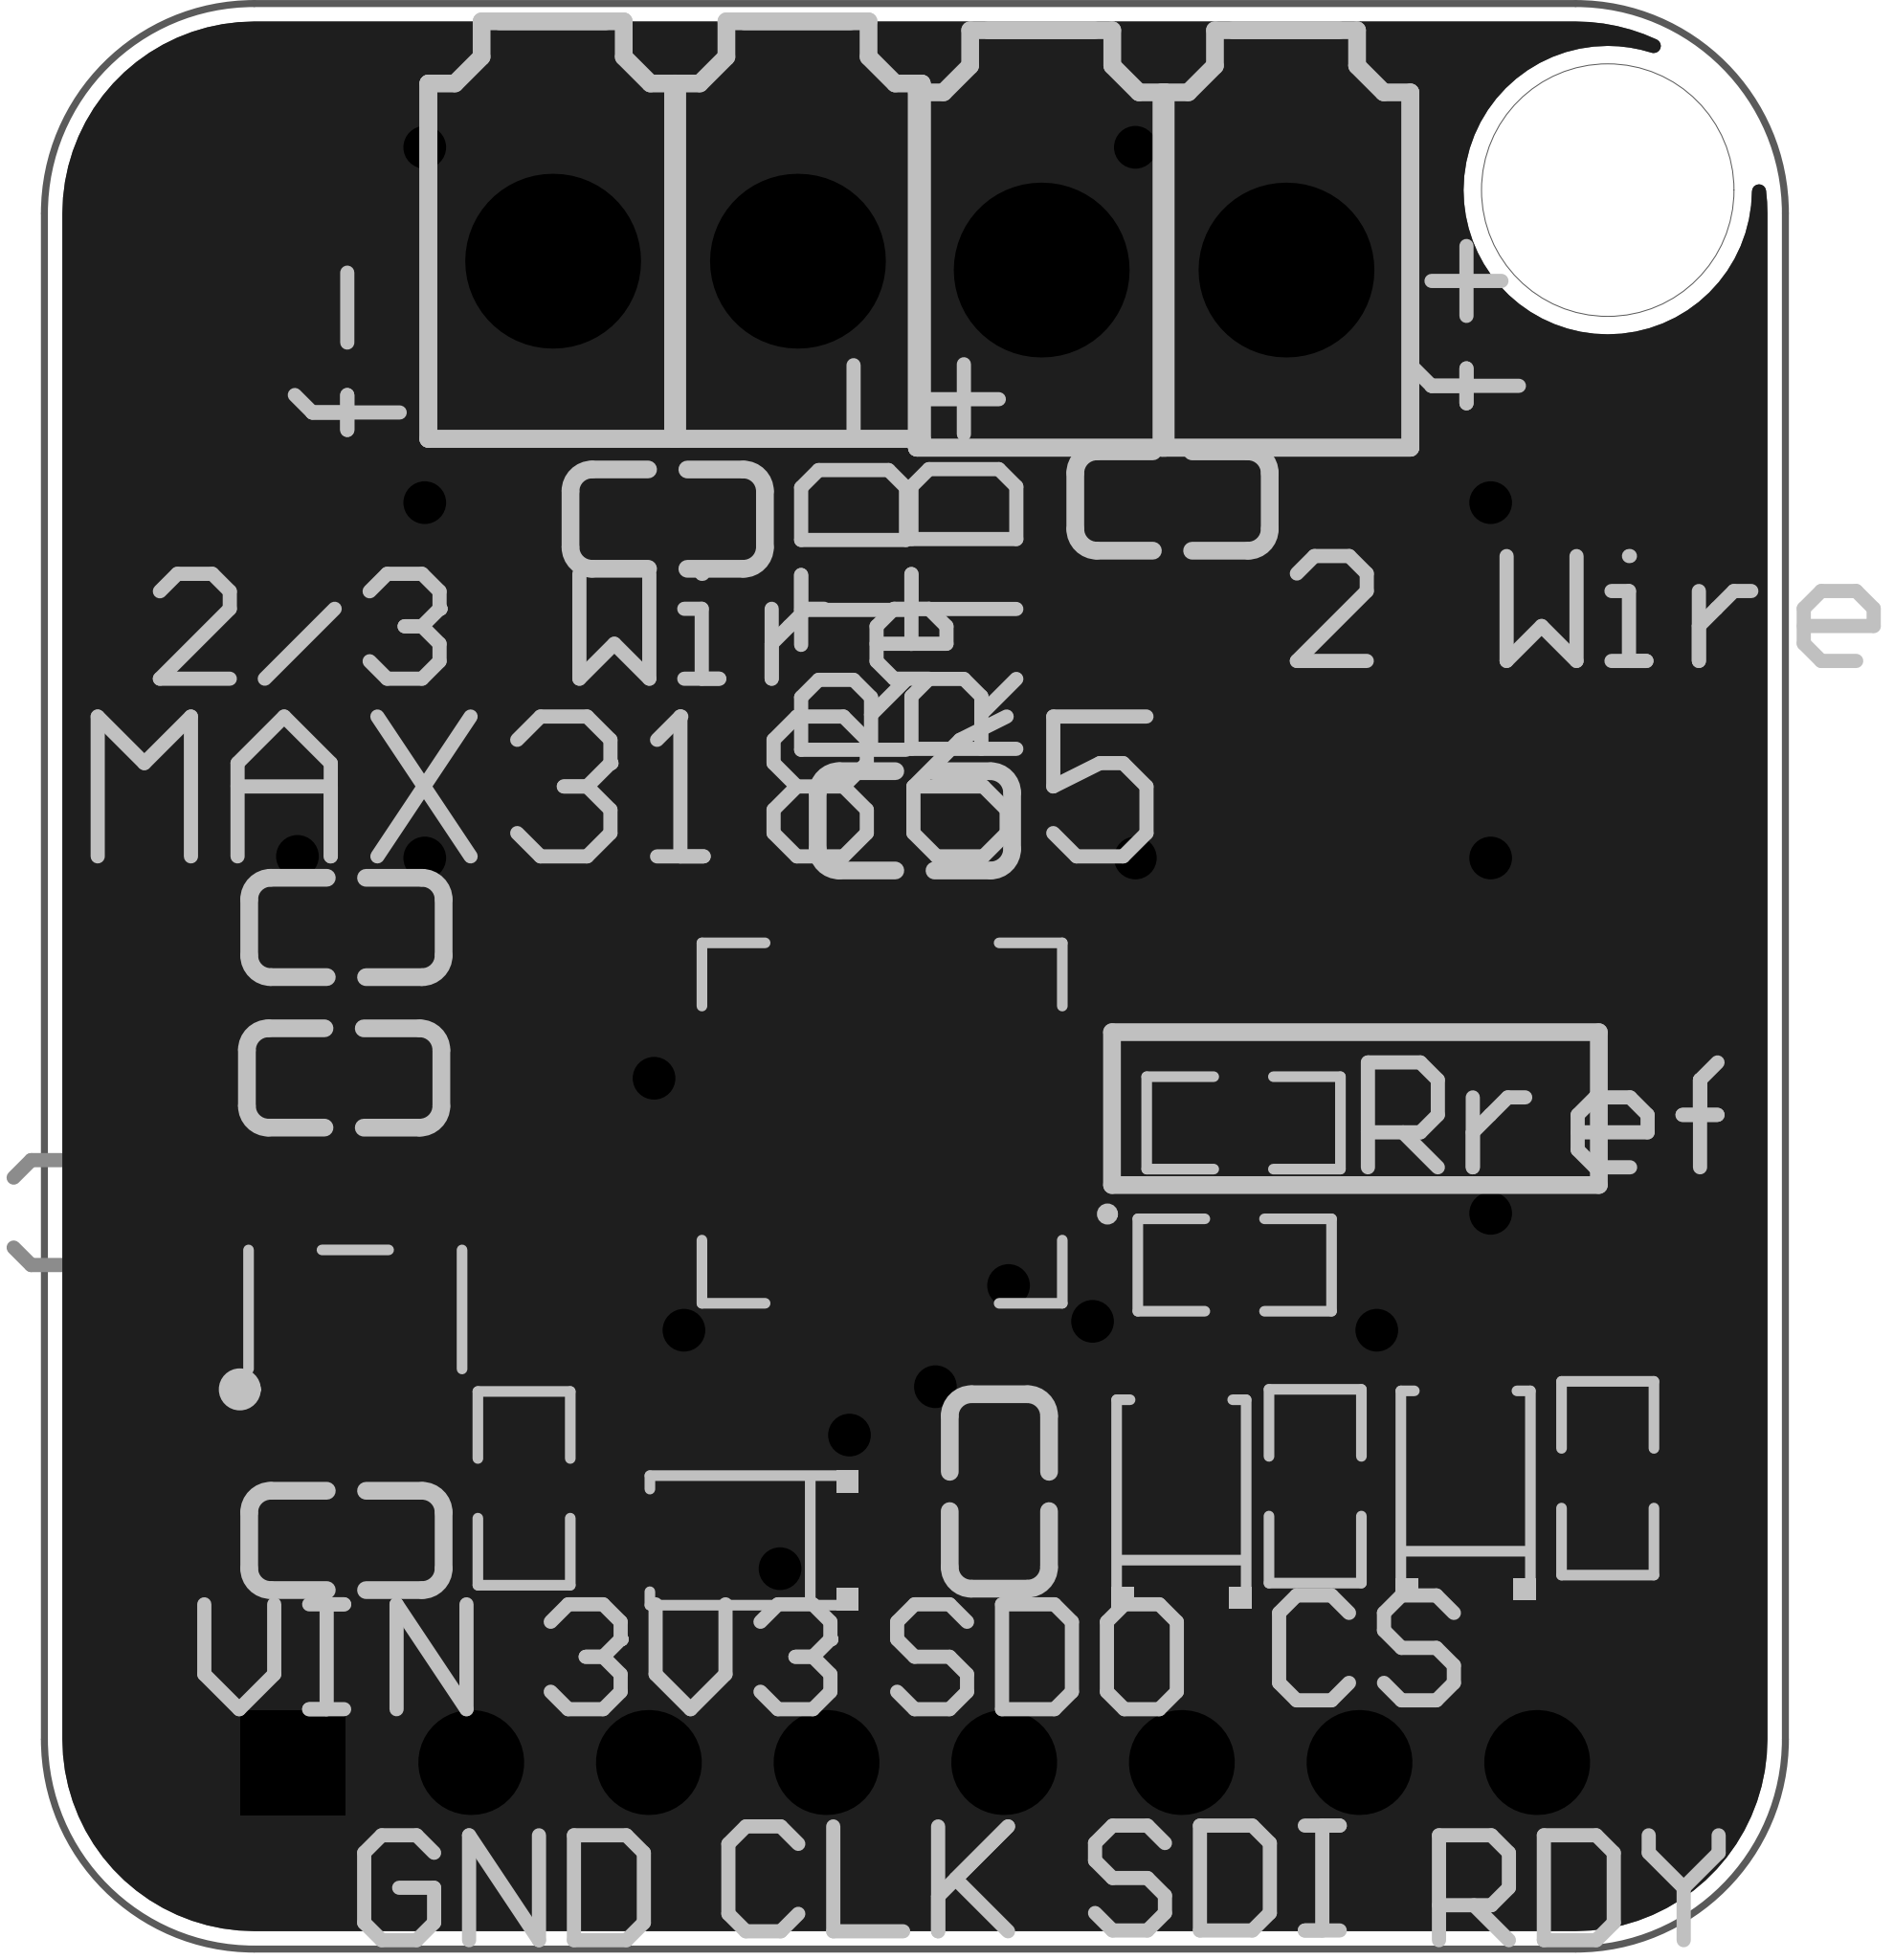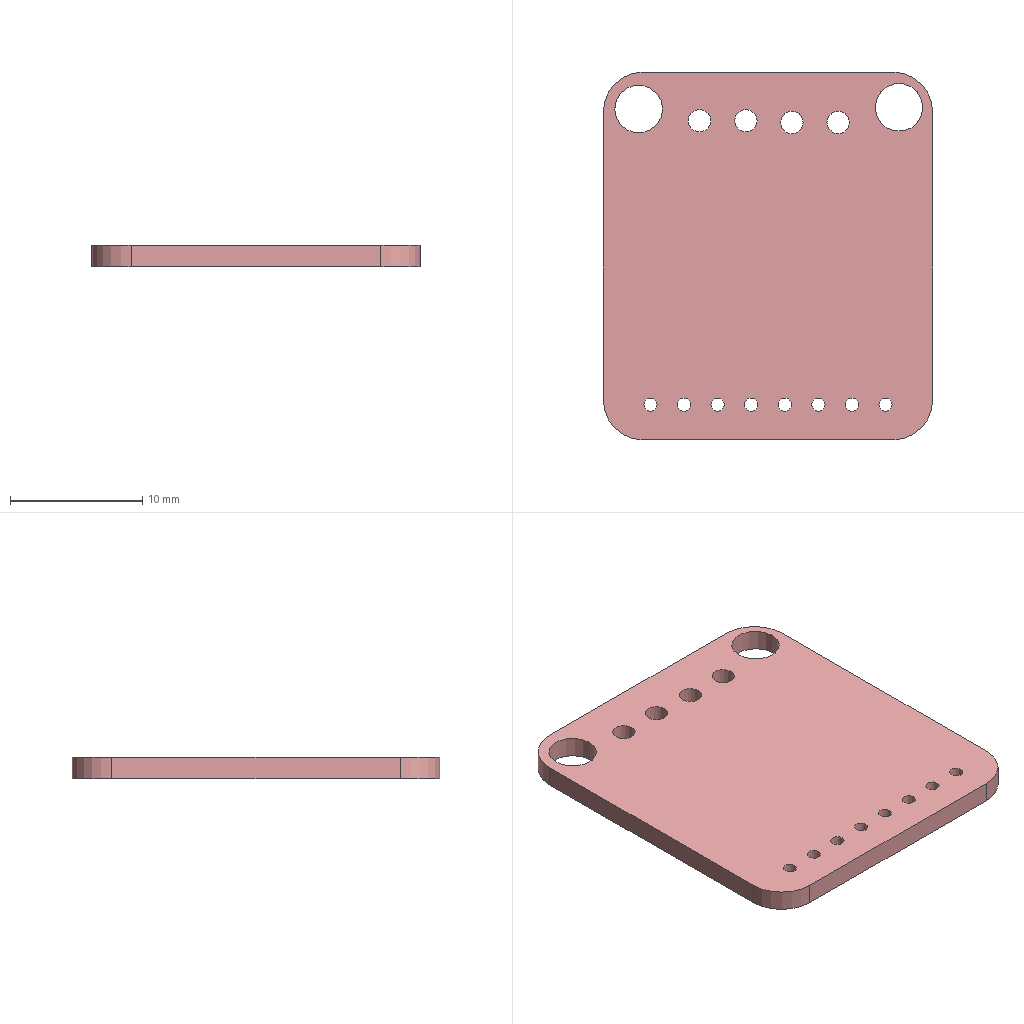Circuit board layout | Altium Designer | box 24.9 x 27.8 x 1.6 mm
Layer stack:
# Altium Designer layer stack of  (unit mm; dielectric type: 0 none, 1 core, 2 prepreg, 3 surface material)
index,name,kind,layer,copper_thickness_mm,dielectric_type,dielectric_thickness_mm,dielectric_material,dielectric_constant
0,Top Paste Mask Layer,other,,,,,,
1,Top Silkscreen Layer,other,,,,,,
2,Top Solder Mask Layer,dielectric,,,3,0.01,,3.3
3,Top Layer,copper,Top Layer,0.035,,,,
4,Dielectric1,dielectric,,,3,1.51,FR4,4.5
5,Bottom Layer,copper,Bottom Layer,0.035,,,,
6,Bottom Solder Mask Layer,dielectric,,,3,0.01,,3.3
7,Bottom Silkscreen Layer,other,,,,,,
8,Bottom Paste Mask Layer,other,,,,,,
# drill layer pairs: low layer,high layer
drill_pair,Top Layer,Bottom Layer
Part placement:
Designator,Comment,Layer,Footprint,Center-X(mm),Center-Y(mm),Rotation
C1,100nF,TopLayer,C0603,84.709,93.472,180
C2,100nF,TopLayer,C0603,94.045,85.409,90
C3,10uF,TopLayer,C0603,84.709,84.709,180
C4,10uF,TopLayer,C0603,84.676,91.32,180
C5,100nF,TopLayer,C0603,92.837,94.996,0
D1,1N4148W,TopLayer,SOD-123F_L2.7-W1.6-LS3.8-RD,90.424,84.709,180
D2,1N4148W,TopLayer,SOD-123F_L2.7-W1.6-LS3.8-RD,96.647,85.344,90
D3,1N4148W,TopLayer,SOD-123F_L2.7-W1.6-LS3.8-RD,100.711,85.471,90
H1,,TopLayer,HDR-TH_8P-P2.54-V-M,92.837,81.534,0
C6,100nF,TopLayer,C0603,96.52,99.568,0
C7,100nF,TopLayer,C0603,89.303,99.309,0
R1,10K,TopLayer,R0603,97.409,88.646,0
R2,10K,TopLayer,R0603,98.56,85.484,270
R3,10K,TopLayer,R0603,102.743,85.598,270
R4,10K,TopLayer,R0603,87.249,85.454,270
R5,10K,TopLayer,R0603,97.536,90.678,180
U1,MAX3186,TopLayer,QFN-20_L5.0-W5.0-P0.65-BL-EP,92.368,90.675,90
U2,MIC5225-3.3,TopLayer,SOT-23-5_L3.0-W1.7-P0.95-LS2.8-BL,84.836,88.011,0
Q1,,TopLayer,S8550P_SOT,98.753,95.503,90
U3,KF2EDGJVC-3.5-2P,TopLayer,CONN-TH_2P-P3.50_KEFA_KF2EDGJVC-3.5-2P,96.393,102.87,0
U4,KF2EDGJVC-3.5-2P,TopLayer,CONN-TH_2P-P3.50_KEFA_KF2EDGJVC-3.5-2P,89.408,102.997,0
Pad and via stacks:
# Altium Designer via and pad stacks of  (unit mm). Each distinct definition once, with the count of objects using it.
# via: kind,start_layer,end_layer,hole_mm,diameter_mm,mode(0 simple;1 top-mid-bottom;2 full stack),diameter_per_layer,count,example_net
# pad: kind,layer,hole_mm,hole_type(0 round;1 square;2 slot),plating,top_size,top_shape(1 round;2 rect;3 octagon;9 rounded rect),mid_size,bottom_size,mode,footprint,size_per_layer,count,example
pad,Top Layer,0,0,plated,0.8x0.9,2,0.8x0.9,0.8x0.9,0,C0603,,14,C1.2
pad,Top Layer,0,0,plated,1.1x1,2,1.1x1,1.1x1,0,SOD-123F_L2.7-W1.6-LS3.8-RD,,6,D1.2
pad,Top Layer,0,0,plated,0.8065x0.864,2,0.8065x0.864,0.8065x0.864,0,R0603,,10,R1.2
pad,Top Layer,0,0,plated,0.364x0.847,1,0.364x0.847,0.364x0.847,0,QFN-20_L5.0-W5.0-P0.65-BL-EP,,10,U1.1
pad,Top Layer,0,0,plated,0.847x0.364,1,0.847x0.364,0.847x0.364,0,QFN-20_L5.0-W5.0-P0.65-BL-EP,,10,U1.6
pad,Top Layer,0,0,plated,3.25x3.25,2,3.25x3.25,3.25x3.25,0,QFN-20_L5.0-W5.0-P0.65-BL-EP,,1,U1.21
pad,Top Layer,0,0,plated,0.49x1.157,2,0.49x1.157,0.49x1.157,0,SOT-23-5_L3.0-W1.7-P0.95-LS2.8-BL,,3,U2.1
pad,Top Layer,0,0,plated,0.49x1.175,2,0.49x1.175,0.49x1.175,0,SOT-23-5_L3.0-W1.7-P0.95-LS2.8-BL,,2,U2.4
pad,Top Layer,0,0,plated,0.701x1.25,2,0.701x1.25,0.701x1.25,0,S8550P_SOT,,3,Q1.1
pad,Multi-Layer,1,0,plated,1.5x1.5,2,1.5x1.5,1.5x1.5,0,HDR-TH_8P-P2.54-V-M,,1,H1.1
pad,Multi-Layer,1,0,plated,1.5x1.5,1,1.5x1.5,1.5x1.5,0,HDR-TH_8P-P2.54-V-M,,7,H1.2
pad,Multi-Layer,1.7,0,plated,2.5x2.5,1,2.5x2.5,2.5x2.5,0,CONN-TH_2P-P3.50_KEFA_KF2EDGJVC-3.5-2P,,4,U3.1
via,Top Layer,Bottom Layer,0.3048,0.61,0,,17,$1N345
via,Top Layer,Bottom Layer,0.3048,0.6096,0,,4,
Copper pours:
name,layer,net,type(0 solid;1 hatched;2 none)
Top Layer-GND,Top Layer,GND,0
Bottom Layer-GND,Bottom Layer,GND,0